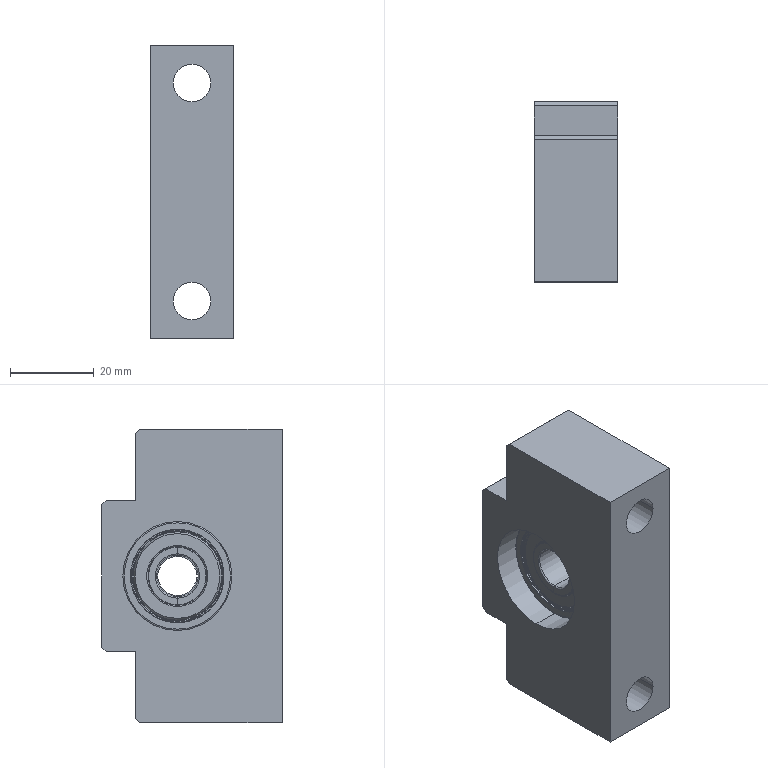Part | STEP file | 001-008-LEB51-12 | 3 solids | 186 faces | box 20 x 43 x 70 mm | volume 40674 mm3 | cylinder 56 | torus 48 | cone 48 | plane 34 | commonest cylinder face diameters 1 x4 2.207 x4 9 x4 13.3 x4 13.9 x4 14 x4